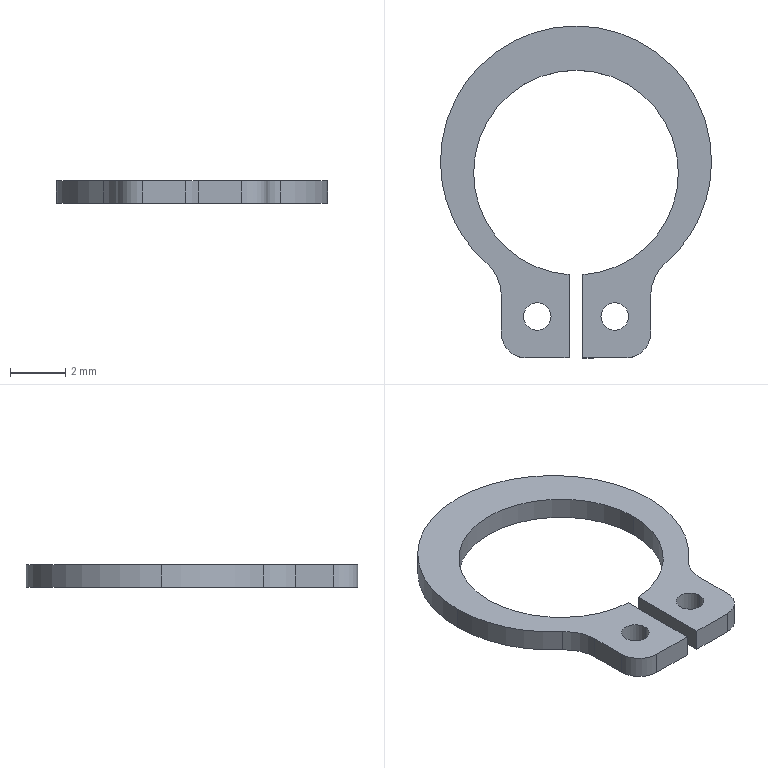Part | SolidWorks | features BaseBody 1 | 1 solid | 22 faces | box 9.8 x 12 x 0.8 mm | volume 33.948 mm3 | cylinder 14 | plane 8 | commonest cylinder face diameters 1 x4 7.4 x3 9.8 x3 1.8 x2 3 x2
STEP:
#1=CARTESIAN_POINT('',(-0.9,-5.2,-0.4));
#2=VERTEX_POINT('',#1);
#3=CARTESIAN_POINT('',(-1.9,-5.2,-0.4));
#4=VERTEX_POINT('',#3);
#5=CARTESIAN_POINT('',(-1.4,-5.2,-0.4));
#6=DIRECTION('',(0.,0.,-1.));
#7=DIRECTION('',(1.,0.,0.));
#8=AXIS2_PLACEMENT_3D('',#5,#6,#7);
#9=CIRCLE('',#8,0.5);
#10=EDGE_CURVE('',#2,#4,#9,.T.);
#11=ORIENTED_EDGE('',*,*,#10,.T.);
#12=CARTESIAN_POINT('',(-1.9,-5.2,0.4));
#13=VERTEX_POINT('',#12);
#14=CARTESIAN_POINT('',(-1.9,-5.2,0.4));
#15=DIRECTION('',(0.,0.,1.));
#16=VECTOR('',#15,1000.);
#17=LINE('',#14,#16);
#18=EDGE_CURVE('',#4,#13,#17,.T.);
#19=ORIENTED_EDGE('',*,*,#18,.T.);
#20=CARTESIAN_POINT('',(-0.9,-5.2,0.4));
#21=VERTEX_POINT('',#20);
#22=CARTESIAN_POINT('',(-1.4,-5.2,0.4));
#23=DIRECTION('',(0.,0.,-1.));
#24=DIRECTION('',(1.,0.,0.));
#25=AXIS2_PLACEMENT_3D('',#22,#23,#24);
#26=CIRCLE('',#25,0.5);
#27=EDGE_CURVE('',#21,#13,#26,.T.);
#28=ORIENTED_EDGE('',*,*,#27,.F.);
#29=CARTESIAN_POINT('',(-0.9,-5.2,0.4));
#30=DIRECTION('',(0.,0.,1.));
#31=VECTOR('',#30,1000.);
#32=LINE('',#29,#31);
#33=EDGE_CURVE('',#2,#21,#32,.T.);
#34=ORIENTED_EDGE('',*,*,#33,.F.);
#35=EDGE_LOOP('',(#11,#19,#28,#34));
#36=FACE_OUTER_BOUND('',#35,.T.);
#37=CARTESIAN_POINT('',(-1.4,-5.2,0.4));
#38=DIRECTION('',(0.,0.,1.));
#39=DIRECTION('',(1.,0.,0.));
#40=AXIS2_PLACEMENT_3D('',#37,#38,#39);
#41=CYLINDRICAL_SURFACE('',#40,0.5);
#42=ADVANCED_FACE('',(#36),#41,.F.);
#43=CARTESIAN_POINT('',(-0.25,-3.692,-0.4));
#44=VERTEX_POINT('',#43);
#45=CARTESIAN_POINT('',(-3.7,0.,-0.4));
#46=VERTEX_POINT('',#45);
#47=CARTESIAN_POINT('',(0.,0.,-0.4));
#48=DIRECTION('',(0.,0.,-1.));
#49=DIRECTION('',(1.,0.,0.));
#50=AXIS2_PLACEMENT_3D('',#47,#48,#49);
#51=CIRCLE('',#50,3.7);
#52=EDGE_CURVE('',#44,#46,#51,.T.);
#53=ORIENTED_EDGE('',*,*,#52,.T.);
#54=CARTESIAN_POINT('',(-3.7,0.,0.4));
#55=VERTEX_POINT('',#54);
#56=CARTESIAN_POINT('',(-3.7,0.,0.4));
#57=DIRECTION('',(0.,0.,1.));
#58=VECTOR('',#57,1000.);
#59=LINE('',#56,#58);
#60=EDGE_CURVE('',#46,#55,#59,.T.);
#61=ORIENTED_EDGE('',*,*,#60,.T.);
#62=CARTESIAN_POINT('',(-0.25,-3.692,0.4));
#63=VERTEX_POINT('',#62);
#64=CARTESIAN_POINT('',(0.,0.,0.4));
#65=DIRECTION('',(0.,0.,-1.));
#66=DIRECTION('',(1.,0.,0.));
#67=AXIS2_PLACEMENT_3D('',#64,#65,#66);
#68=CIRCLE('',#67,3.7);
#69=EDGE_CURVE('',#63,#55,#68,.T.);
#70=ORIENTED_EDGE('',*,*,#69,.F.);
#71=CARTESIAN_POINT('',(-0.25,-3.692,0.4));
#72=DIRECTION('',(0.,0.,1.));
#73=VECTOR('',#72,1000.);
#74=LINE('',#71,#73);
#75=EDGE_CURVE('',#44,#63,#74,.T.);
#76=ORIENTED_EDGE('',*,*,#75,.F.);
#77=EDGE_LOOP('',(#53,#61,#70,#76));
#78=FACE_OUTER_BOUND('',#77,.T.);
#79=CARTESIAN_POINT('',(0.,0.,0.4));
#80=DIRECTION('',(0.,0.,1.));
#81=DIRECTION('',(1.,0.,0.));
#82=AXIS2_PLACEMENT_3D('',#79,#80,#81);
#83=CYLINDRICAL_SURFACE('',#82,3.7);
#84=ADVANCED_FACE('',(#78),#83,.F.);
#85=ORIENTED_EDGE('',*,*,#60,.F.);
#86=CARTESIAN_POINT('',(3.7,0.,-0.4));
#87=VERTEX_POINT('',#86);
#88=CARTESIAN_POINT('',(0.,0.,-0.4));
#89=DIRECTION('',(0.,0.,-1.));
#90=DIRECTION('',(1.,0.,0.));
#91=AXIS2_PLACEMENT_3D('',#88,#89,#90);
#92=CIRCLE('',#91,3.7);
#93=EDGE_CURVE('',#46,#87,#92,.T.);
#94=ORIENTED_EDGE('',*,*,#93,.T.);
#95=CARTESIAN_POINT('',(3.7,0.,0.4));
#96=VERTEX_POINT('',#95);
#97=CARTESIAN_POINT('',(3.7,0.,0.4));
#98=DIRECTION('',(0.,0.,1.));
#99=VECTOR('',#98,1000.);
#100=LINE('',#97,#99);
#101=EDGE_CURVE('',#87,#96,#100,.T.);
#102=ORIENTED_EDGE('',*,*,#101,.T.);
#103=CARTESIAN_POINT('',(0.,0.,0.4));
#104=DIRECTION('',(0.,0.,-1.));
#105=DIRECTION('',(1.,0.,0.));
#106=AXIS2_PLACEMENT_3D('',#103,#104,#105);
#107=CIRCLE('',#106,3.7);
#108=EDGE_CURVE('',#55,#96,#107,.T.);
#109=ORIENTED_EDGE('',*,*,#108,.F.);
#110=EDGE_LOOP('',(#85,#94,#102,#109));
#111=FACE_OUTER_BOUND('',#110,.T.);
#112=CARTESIAN_POINT('',(0.,0.,0.4));
#113=DIRECTION('',(0.,0.,1.));
#114=DIRECTION('',(1.,0.,0.));
#115=AXIS2_PLACEMENT_3D('',#112,#113,#114);
#116=CYLINDRICAL_SURFACE('',#115,3.7);
#117=ADVANCED_FACE('',(#111),#116,.F.);
#118=CARTESIAN_POINT('',(4.9,0.4,-0.4));
#119=VERTEX_POINT('',#118);
#120=CARTESIAN_POINT('',(-4.9,0.4,-0.4));
#121=VERTEX_POINT('',#120);
#122=CARTESIAN_POINT('',(0.,0.4,-0.4));
#123=DIRECTION('',(0.,0.,1.));
#124=DIRECTION('',(1.,0.,0.));
#125=AXIS2_PLACEMENT_3D('',#122,#123,#124);
#126=CIRCLE('',#125,4.9);
#127=EDGE_CURVE('',#119,#121,#126,.T.);
#128=ORIENTED_EDGE('',*,*,#127,.T.);
#129=CARTESIAN_POINT('',(-4.9,0.4,0.4));
#130=VERTEX_POINT('',#129);
#131=CARTESIAN_POINT('',(-4.9,0.4,0.4));
#132=DIRECTION('',(0.,0.,1.));
#133=VECTOR('',#132,1000.);
#134=LINE('',#131,#133);
#135=EDGE_CURVE('',#121,#130,#134,.T.);
#136=ORIENTED_EDGE('',*,*,#135,.T.);
#137=CARTESIAN_POINT('',(4.9,0.4,0.4));
#138=VERTEX_POINT('',#137);
#139=CARTESIAN_POINT('',(0.,0.4,0.4));
#140=DIRECTION('',(0.,0.,-1.));
#141=DIRECTION('',(1.,0.,0.));
#142=AXIS2_PLACEMENT_3D('',#139,#140,#141);
#143=CIRCLE('',#142,4.9);
#144=EDGE_CURVE('',#130,#138,#143,.T.);
#145=ORIENTED_EDGE('',*,*,#144,.T.);
#146=CARTESIAN_POINT('',(4.9,0.4,0.4));
#147=DIRECTION('',(0.,0.,1.));
#148=VECTOR('',#147,1000.);
#149=LINE('',#146,#148);
#150=EDGE_CURVE('',#119,#138,#149,.T.);
#151=ORIENTED_EDGE('',*,*,#150,.F.);
#152=EDGE_LOOP('',(#128,#136,#145,#151));
#153=FACE_OUTER_BOUND('',#152,.T.);
#154=CARTESIAN_POINT('',(0.,0.4,0.4));
#155=DIRECTION('',(0.,0.,1.));
#156=DIRECTION('',(1.,0.,0.));
#157=AXIS2_PLACEMENT_3D('',#154,#155,#156);
#158=CYLINDRICAL_SURFACE('',#157,4.9);
#159=ADVANCED_FACE('',(#153),#158,.T.);
#160=CARTESIAN_POINT('',(3.216,-3.297,-0.4));
#161=VERTEX_POINT('',#160);
#162=CARTESIAN_POINT('',(0.,0.4,-0.4));
#163=DIRECTION('',(0.,0.,1.));
#164=DIRECTION('',(1.,0.,0.));
#165=AXIS2_PLACEMENT_3D('',#162,#163,#164);
#166=CIRCLE('',#165,4.9);
#167=EDGE_CURVE('',#161,#119,#166,.T.);
#168=ORIENTED_EDGE('',*,*,#167,.T.);
#169=ORIENTED_EDGE('',*,*,#150,.T.);
#170=CARTESIAN_POINT('',(3.216,-3.297,0.4));
#171=VERTEX_POINT('',#170);
#172=CARTESIAN_POINT('',(0.,0.4,0.4));
#173=DIRECTION('',(0.,0.,-1.));
#174=DIRECTION('',(1.,0.,0.));
#175=AXIS2_PLACEMENT_3D('',#172,#173,#174);
#176=CIRCLE('',#175,4.9);
#177=EDGE_CURVE('',#138,#171,#176,.T.);
#178=ORIENTED_EDGE('',*,*,#177,.T.);
#179=CARTESIAN_POINT('',(3.216,-3.297,0.4));
#180=DIRECTION('',(0.,0.,-1.));
#181=VECTOR('',#180,1000.);
#182=LINE('',#179,#181);
#183=EDGE_CURVE('',#171,#161,#182,.T.);
#184=ORIENTED_EDGE('',*,*,#183,.T.);
#185=EDGE_LOOP('',(#168,#169,#178,#184));
#186=FACE_OUTER_BOUND('',#185,.T.);
#187=CARTESIAN_POINT('',(0.,0.4,0.4));
#188=DIRECTION('',(0.,0.,1.));
#189=DIRECTION('',(1.,0.,0.));
#190=AXIS2_PLACEMENT_3D('',#187,#188,#189);
#191=CYLINDRICAL_SURFACE('',#190,4.9);
#192=ADVANCED_FACE('',(#186),#191,.T.);
#193=CARTESIAN_POINT('',(1.9,-5.2,-0.4));
#194=VERTEX_POINT('',#193);
#195=CARTESIAN_POINT('',(0.9,-5.2,-0.4));
#196=VERTEX_POINT('',#195);
#197=CARTESIAN_POINT('',(1.4,-5.2,-0.4));
#198=DIRECTION('',(0.,0.,-1.));
#199=DIRECTION('',(1.,0.,0.));
#200=AXIS2_PLACEMENT_3D('',#197,#198,#199);
#201=CIRCLE('',#200,0.5);
#202=EDGE_CURVE('',#194,#196,#201,.T.);
#203=ORIENTED_EDGE('',*,*,#202,.T.);
#204=CARTESIAN_POINT('',(0.9,-5.2,0.4));
#205=VERTEX_POINT('',#204);
#206=CARTESIAN_POINT('',(0.9,-5.2,0.4));
#207=DIRECTION('',(0.,0.,1.));
#208=VECTOR('',#207,1000.);
#209=LINE('',#206,#208);
#210=EDGE_CURVE('',#196,#205,#209,.T.);
#211=ORIENTED_EDGE('',*,*,#210,.T.);
#212=CARTESIAN_POINT('',(1.9,-5.2,0.4));
#213=VERTEX_POINT('',#212);
#214=CARTESIAN_POINT('',(1.4,-5.2,0.4));
#215=DIRECTION('',(0.,0.,-1.));
#216=DIRECTION('',(1.,0.,0.));
#217=AXIS2_PLACEMENT_3D('',#214,#215,#216);
#218=CIRCLE('',#217,0.5);
#219=EDGE_CURVE('',#213,#205,#218,.T.);
#220=ORIENTED_EDGE('',*,*,#219,.F.);
#221=CARTESIAN_POINT('',(1.9,-5.2,0.4));
#222=DIRECTION('',(0.,0.,1.));
#223=VECTOR('',#222,1000.);
#224=LINE('',#221,#223);
#225=EDGE_CURVE('',#194,#213,#224,.T.);
#226=ORIENTED_EDGE('',*,*,#225,.F.);
#227=EDGE_LOOP('',(#203,#211,#220,#226));
#228=FACE_OUTER_BOUND('',#227,.T.);
#229=CARTESIAN_POINT('',(1.4,-5.2,0.4));
#230=DIRECTION('',(0.,0.,1.));
#231=DIRECTION('',(1.,0.,0.));
#232=AXIS2_PLACEMENT_3D('',#229,#230,#231);
#233=CYLINDRICAL_SURFACE('',#232,0.5);
#234=ADVANCED_FACE('',(#228),#233,.F.);
#235=ORIENTED_EDGE('',*,*,#10,.F.);
#236=CARTESIAN_POINT('',(-1.4,-5.2,-0.4));
#237=DIRECTION('',(0.,0.,-1.));
#238=DIRECTION('',(1.,0.,0.));
#239=AXIS2_PLACEMENT_3D('',#236,#237,#238);
#240=CIRCLE('',#239,0.5);
#241=EDGE_CURVE('',#4,#2,#240,.T.);
#242=ORIENTED_EDGE('',*,*,#241,.F.);
#243=EDGE_LOOP('',(#235,#242));
#244=FACE_BOUND('',#243,.T.);
#245=CARTESIAN_POINT('',(2.7,-5.8,-0.4));
#246=VERTEX_POINT('',#245);
#247=CARTESIAN_POINT('',(2.7,-4.429,-0.4));
#248=VERTEX_POINT('',#247);
#249=CARTESIAN_POINT('',(2.7,-4.429,-0.4));
#250=DIRECTION('',(0.,1.,0.));
#251=VECTOR('',#250,1000.);
#252=LINE('',#249,#251);
#253=EDGE_CURVE('',#246,#248,#252,.T.);
#254=ORIENTED_EDGE('',*,*,#253,.F.);
#255=CARTESIAN_POINT('',(1.8,-6.7,-0.4));
#256=VERTEX_POINT('',#255);
#257=CARTESIAN_POINT('',(1.8,-5.8,-0.4));
#258=DIRECTION('',(0.,0.,1.));
#259=DIRECTION('',(1.,0.,0.));
#260=AXIS2_PLACEMENT_3D('',#257,#258,#259);
#261=CIRCLE('',#260,0.9);
#262=EDGE_CURVE('',#256,#246,#261,.T.);
#263=ORIENTED_EDGE('',*,*,#262,.F.);
#264=CARTESIAN_POINT('',(0.25,-6.7,-0.4));
#265=VERTEX_POINT('',#264);
#266=CARTESIAN_POINT('',(4.2,-6.7,-0.4));
#267=DIRECTION('',(1.,0.,0.));
#268=VECTOR('',#267,1000.);
#269=LINE('',#266,#268);
#270=EDGE_CURVE('',#265,#256,#269,.T.);
#271=ORIENTED_EDGE('',*,*,#270,.F.);
#272=CARTESIAN_POINT('',(0.25,-3.692,-0.4));
#273=VERTEX_POINT('',#272);
#274=CARTESIAN_POINT('',(0.25,-4.429,-0.4));
#275=DIRECTION('',(0.,-1.,0.));
#276=VECTOR('',#275,1000.);
#277=LINE('',#274,#276);
#278=EDGE_CURVE('',#273,#265,#277,.T.);
#279=ORIENTED_EDGE('',*,*,#278,.F.);
#280=CARTESIAN_POINT('',(0.,0.,-0.4));
#281=DIRECTION('',(0.,0.,-1.));
#282=DIRECTION('',(1.,0.,0.));
#283=AXIS2_PLACEMENT_3D('',#280,#281,#282);
#284=CIRCLE('',#283,3.7);
#285=EDGE_CURVE('',#87,#273,#284,.T.);
#286=ORIENTED_EDGE('',*,*,#285,.F.);
#287=ORIENTED_EDGE('',*,*,#93,.F.);
#288=ORIENTED_EDGE('',*,*,#52,.F.);
#289=CARTESIAN_POINT('',(-0.25,-6.7,-0.4));
#290=VERTEX_POINT('',#289);
#291=CARTESIAN_POINT('',(-0.25,-4.429,-0.4));
#292=DIRECTION('',(0.,1.,0.));
#293=VECTOR('',#292,1000.);
#294=LINE('',#291,#293);
#295=EDGE_CURVE('',#290,#44,#294,.T.);
#296=ORIENTED_EDGE('',*,*,#295,.F.);
#297=CARTESIAN_POINT('',(-1.8,-6.7,-0.4));
#298=VERTEX_POINT('',#297);
#299=CARTESIAN_POINT('',(4.2,-6.7,-0.4));
#300=DIRECTION('',(1.,0.,0.));
#301=VECTOR('',#300,1000.);
#302=LINE('',#299,#301);
#303=EDGE_CURVE('',#298,#290,#302,.T.);
#304=ORIENTED_EDGE('',*,*,#303,.F.);
#305=CARTESIAN_POINT('',(-2.7,-5.8,-0.4));
#306=VERTEX_POINT('',#305);
#307=CARTESIAN_POINT('',(-1.8,-5.8,-0.4));
#308=DIRECTION('',(0.,0.,1.));
#309=DIRECTION('',(1.,0.,0.));
#310=AXIS2_PLACEMENT_3D('',#307,#308,#309);
#311=CIRCLE('',#310,0.9);
#312=EDGE_CURVE('',#306,#298,#311,.T.);
#313=ORIENTED_EDGE('',*,*,#312,.F.);
#314=CARTESIAN_POINT('',(-2.7,-4.429,-0.4));
#315=VERTEX_POINT('',#314);
#316=CARTESIAN_POINT('',(-2.7,-4.429,-0.4));
#317=DIRECTION('',(0.,-1.,0.));
#318=VECTOR('',#317,1000.);
#319=LINE('',#316,#318);
#320=EDGE_CURVE('',#315,#306,#319,.T.);
#321=ORIENTED_EDGE('',*,*,#320,.F.);
#322=CARTESIAN_POINT('',(-3.216,-3.297,-0.4));
#323=VERTEX_POINT('',#322);
#324=CARTESIAN_POINT('',(-4.2,-4.429,-0.4));
#325=DIRECTION('',(0.,0.,-1.));
#326=DIRECTION('',(1.,0.,0.));
#327=AXIS2_PLACEMENT_3D('',#324,#325,#326);
#328=CIRCLE('',#327,1.5);
#329=EDGE_CURVE('',#323,#315,#328,.T.);
#330=ORIENTED_EDGE('',*,*,#329,.F.);
#331=CARTESIAN_POINT('',(0.,0.4,-0.4));
#332=DIRECTION('',(0.,0.,1.));
#333=DIRECTION('',(1.,0.,0.));
#334=AXIS2_PLACEMENT_3D('',#331,#332,#333);
#335=CIRCLE('',#334,4.9);
#336=EDGE_CURVE('',#121,#323,#335,.T.);
#337=ORIENTED_EDGE('',*,*,#336,.F.);
#338=ORIENTED_EDGE('',*,*,#127,.F.);
#339=ORIENTED_EDGE('',*,*,#167,.F.);
#340=CARTESIAN_POINT('',(4.2,-4.429,-0.4));
#341=DIRECTION('',(0.,0.,-1.));
#342=DIRECTION('',(1.,0.,0.));
#343=AXIS2_PLACEMENT_3D('',#340,#341,#342);
#344=CIRCLE('',#343,1.5);
#345=EDGE_CURVE('',#248,#161,#344,.T.);
#346=ORIENTED_EDGE('',*,*,#345,.F.);
#347=EDGE_LOOP('',(#254,#263,#271,#279,#286,#287,#288,#296,#304,#313,#321,#330,#337,#338,#339,#346));
#348=FACE_OUTER_BOUND('',#347,.T.);
#349=ORIENTED_EDGE('',*,*,#202,.F.);
#350=CARTESIAN_POINT('',(1.4,-5.2,-0.4));
#351=DIRECTION('',(0.,0.,-1.));
#352=DIRECTION('',(1.,0.,0.));
#353=AXIS2_PLACEMENT_3D('',#350,#351,#352);
#354=CIRCLE('',#353,0.5);
#355=EDGE_CURVE('',#196,#194,#354,.T.);
#356=ORIENTED_EDGE('',*,*,#355,.F.);
#357=EDGE_LOOP('',(#349,#356));
#358=FACE_BOUND('',#357,.T.);
#359=CARTESIAN_POINT('',(4.2,-4.429,-0.4));
#360=DIRECTION('',(0.,0.,1.));
#361=DIRECTION('',(1.,0.,0.));
#362=AXIS2_PLACEMENT_3D('',#359,#360,#361);
#363=PLANE('',#362);
#364=ADVANCED_FACE('',(#244,#348,#358),#363,.F.);
#365=ORIENTED_EDGE('',*,*,#18,.F.);
#366=ORIENTED_EDGE('',*,*,#241,.T.);
#367=ORIENTED_EDGE('',*,*,#33,.T.);
#368=CARTESIAN_POINT('',(-1.4,-5.2,0.4));
#369=DIRECTION('',(0.,0.,-1.));
#370=DIRECTION('',(1.,0.,0.));
#371=AXIS2_PLACEMENT_3D('',#368,#369,#370);
#372=CIRCLE('',#371,0.5);
#373=EDGE_CURVE('',#13,#21,#372,.T.);
#374=ORIENTED_EDGE('',*,*,#373,.F.);
#375=EDGE_LOOP('',(#365,#366,#367,#374));
#376=FACE_OUTER_BOUND('',#375,.T.);
#377=CARTESIAN_POINT('',(-1.4,-5.2,0.4));
#378=DIRECTION('',(0.,0.,1.));
#379=DIRECTION('',(1.,0.,0.));
#380=AXIS2_PLACEMENT_3D('',#377,#378,#379);
#381=CYLINDRICAL_SURFACE('',#380,0.5);
#382=ADVANCED_FACE('',(#376),#381,.F.);
#383=ORIENTED_EDGE('',*,*,#183,.F.);
#384=CARTESIAN_POINT('',(2.7,-4.429,0.4));
#385=VERTEX_POINT('',#384);
#386=CARTESIAN_POINT('',(4.2,-4.429,0.4));
#387=DIRECTION('',(0.,0.,-1.));
#388=DIRECTION('',(1.,0.,0.));
#389=AXIS2_PLACEMENT_3D('',#386,#387,#388);
#390=CIRCLE('',#389,1.5);
#391=EDGE_CURVE('',#385,#171,#390,.T.);
#392=ORIENTED_EDGE('',*,*,#391,.F.);
#393=CARTESIAN_POINT('',(2.7,-4.429,0.4));
#394=DIRECTION('',(0.,0.,1.));
#395=VECTOR('',#394,1000.);
#396=LINE('',#393,#395);
#397=EDGE_CURVE('',#248,#385,#396,.T.);
#398=ORIENTED_EDGE('',*,*,#397,.F.);
#399=ORIENTED_EDGE('',*,*,#345,.T.);
#400=EDGE_LOOP('',(#383,#392,#398,#399));
#401=FACE_OUTER_BOUND('',#400,.T.);
#402=CARTESIAN_POINT('',(4.2,-4.429,0.4));
#403=DIRECTION('',(0.,0.,1.));
#404=DIRECTION('',(1.,0.,0.));
#405=AXIS2_PLACEMENT_3D('',#402,#403,#404);
#406=CYLINDRICAL_SURFACE('',#405,1.5);
#407=ADVANCED_FACE('',(#401),#406,.F.);
#408=ORIENTED_EDGE('',*,*,#397,.T.);
#409=CARTESIAN_POINT('',(2.7,-5.8,0.4));
#410=VERTEX_POINT('',#409);
#411=CARTESIAN_POINT('',(2.7,-5.8,0.4));
#412=DIRECTION('',(0.,1.,0.));
#413=VECTOR('',#412,1000.);
#414=LINE('',#411,#413);
#415=EDGE_CURVE('',#410,#385,#414,.T.);
#416=ORIENTED_EDGE('',*,*,#415,.F.);
#417=CARTESIAN_POINT('',(2.7,-5.8,0.4));
#418=DIRECTION('',(0.,0.,1.));
#419=VECTOR('',#418,1000.);
#420=LINE('',#417,#419);
#421=EDGE_CURVE('',#246,#410,#420,.T.);
#422=ORIENTED_EDGE('',*,*,#421,.F.);
#423=ORIENTED_EDGE('',*,*,#253,.T.);
#424=EDGE_LOOP('',(#408,#416,#422,#423));
#425=FACE_OUTER_BOUND('',#424,.T.);
#426=CARTESIAN_POINT('',(2.7,-5.8,0.4));
#427=DIRECTION('',(-1.,0.,0.));
#428=DIRECTION('',(0.,0.,1.));
#429=AXIS2_PLACEMENT_3D('',#426,#427,#428);
#430=PLANE('',#429);
#431=ADVANCED_FACE('',(#425),#430,.F.);
#432=CARTESIAN_POINT('',(1.8,-6.7,0.4));
#433=VERTEX_POINT('',#432);
#434=CARTESIAN_POINT('',(1.8,-5.8,0.4));
#435=DIRECTION('',(0.,0.,-1.));
#436=DIRECTION('',(1.,0.,0.));
#437=AXIS2_PLACEMENT_3D('',#434,#435,#436);
#438=CIRCLE('',#437,0.9);
#439=EDGE_CURVE('',#410,#433,#438,.T.);
#440=ORIENTED_EDGE('',*,*,#439,.T.);
#441=CARTESIAN_POINT('',(1.8,-6.7,0.4));
#442=DIRECTION('',(0.,0.,-1.));
#443=VECTOR('',#442,1000.);
#444=LINE('',#441,#443);
#445=EDGE_CURVE('',#433,#256,#444,.T.);
#446=ORIENTED_EDGE('',*,*,#445,.T.);
#447=ORIENTED_EDGE('',*,*,#262,.T.);
#448=ORIENTED_EDGE('',*,*,#421,.T.);
#449=EDGE_LOOP('',(#440,#446,#447,#448));
#450=FACE_OUTER_BOUND('',#449,.T.);
#451=CARTESIAN_POINT('',(1.8,-5.8,0.4));
#452=DIRECTION('',(0.,0.,1.));
#453=DIRECTION('',(1.,0.,0.));
#454=AXIS2_PLACEMENT_3D('',#451,#452,#453);
#455=CYLINDRICAL_SURFACE('',#454,0.9);
#456=ADVANCED_FACE('',(#450),#455,.T.);
#457=ORIENTED_EDGE('',*,*,#445,.F.);
#458=CARTESIAN_POINT('',(0.25,-6.7,0.4));
#459=VERTEX_POINT('',#458);
#460=CARTESIAN_POINT('',(0.25,-6.7,0.4));
#461=DIRECTION('',(1.,0.,0.));
#462=VECTOR('',#461,1000.);
#463=LINE('',#460,#462);
#464=EDGE_CURVE('',#459,#433,#463,.T.);
#465=ORIENTED_EDGE('',*,*,#464,.F.);
#466=CARTESIAN_POINT('',(0.25,-6.7,0.4));
#467=DIRECTION('',(0.,0.,1.));
#468=VECTOR('',#467,1000.);
#469=LINE('',#466,#468);
#470=EDGE_CURVE('',#265,#459,#469,.T.);
#471=ORIENTED_EDGE('',*,*,#470,.F.);
#472=ORIENTED_EDGE('',*,*,#270,.T.);
#473=EDGE_LOOP('',(#457,#465,#471,#472));
#474=FACE_OUTER_BOUND('',#473,.T.);
#475=CARTESIAN_POINT('',(0.25,-6.7,0.4));
#476=DIRECTION('',(0.,1.,0.));
#477=DIRECTION('',(-1.,0.,0.));
#478=AXIS2_PLACEMENT_3D('',#475,#476,#477);
#479=PLANE('',#478);
#480=ADVANCED_FACE('',(#474),#479,.F.);
#481=ORIENTED_EDGE('',*,*,#470,.T.);
#482=CARTESIAN_POINT('',(0.25,-3.692,0.4));
#483=VERTEX_POINT('',#482);
#484=CARTESIAN_POINT('',(0.25,-3.692,0.4));
#485=DIRECTION('',(0.,-1.,0.));
#486=VECTOR('',#485,1000.);
#487=LINE('',#484,#486);
#488=EDGE_CURVE('',#483,#459,#487,.T.);
#489=ORIENTED_EDGE('',*,*,#488,.F.);
#490=CARTESIAN_POINT('',(0.25,-3.692,0.4));
#491=DIRECTION('',(0.,0.,1.));
#492=VECTOR('',#491,1000.);
#493=LINE('',#490,#492);
#494=EDGE_CURVE('',#273,#483,#493,.T.);
#495=ORIENTED_EDGE('',*,*,#494,.F.);
#496=ORIENTED_EDGE('',*,*,#278,.T.);
#497=EDGE_LOOP('',(#481,#489,#495,#496));
#498=FACE_OUTER_BOUND('',#497,.T.);
#499=CARTESIAN_POINT('',(0.25,-3.692,0.4));
#500=DIRECTION('',(1.,0.,0.));
#501=DIRECTION('',(0.,0.,-1.));
#502=AXIS2_PLACEMENT_3D('',#499,#500,#501);
#503=PLANE('',#502);
#504=ADVANCED_FACE('',(#498),#503,.F.);
#505=ORIENTED_EDGE('',*,*,#101,.F.);
#506=ORIENTED_EDGE('',*,*,#285,.T.);
#507=ORIENTED_EDGE('',*,*,#494,.T.);
#508=CARTESIAN_POINT('',(0.,0.,0.4));
#509=DIRECTION('',(0.,0.,-1.));
#510=DIRECTION('',(1.,0.,0.));
#511=AXIS2_PLACEMENT_3D('',#508,#509,#510);
#512=CIRCLE('',#511,3.7);
#513=EDGE_CURVE('',#96,#483,#512,.T.);
#514=ORIENTED_EDGE('',*,*,#513,.F.);
#515=EDGE_LOOP('',(#505,#506,#507,#514));
#516=FACE_OUTER_BOUND('',#515,.T.);
#517=CARTESIAN_POINT('',(0.,0.,0.4));
#518=DIRECTION('',(0.,0.,1.));
#519=DIRECTION('',(1.,0.,0.));
#520=AXIS2_PLACEMENT_3D('',#517,#518,#519);
#521=CYLINDRICAL_SURFACE('',#520,3.7);
#522=ADVANCED_FACE('',(#516),#521,.F.);
#523=ORIENTED_EDGE('',*,*,#75,.T.);
#524=CARTESIAN_POINT('',(-0.25,-6.7,0.4));
#525=VERTEX_POINT('',#524);
#526=CARTESIAN_POINT('',(-0.25,-6.7,0.4));
#527=DIRECTION('',(0.,1.,0.));
#528=VECTOR('',#527,1000.);
#529=LINE('',#526,#528);
#530=EDGE_CURVE('',#525,#63,#529,.T.);
#531=ORIENTED_EDGE('',*,*,#530,.F.);
#532=CARTESIAN_POINT('',(-0.25,-6.7,0.4));
#533=DIRECTION('',(0.,0.,1.));
#534=VECTOR('',#533,1000.);
#535=LINE('',#532,#534);
#536=EDGE_CURVE('',#290,#525,#535,.T.);
#537=ORIENTED_EDGE('',*,*,#536,.F.);
#538=ORIENTED_EDGE('',*,*,#295,.T.);
#539=EDGE_LOOP('',(#523,#531,#537,#538));
#540=FACE_OUTER_BOUND('',#539,.T.);
#541=CARTESIAN_POINT('',(-0.25,-6.7,0.4));
#542=DIRECTION('',(-1.,0.,0.));
#543=DIRECTION('',(0.,0.,1.));
#544=AXIS2_PLACEMENT_3D('',#541,#542,#543);
#545=PLANE('',#544);
#546=ADVANCED_FACE('',(#540),#545,.F.);
#547=ORIENTED_EDGE('',*,*,#536,.T.);
#548=CARTESIAN_POINT('',(-1.8,-6.7,0.4));
#549=VERTEX_POINT('',#548);
#550=CARTESIAN_POINT('',(-1.8,-6.7,0.4));
#551=DIRECTION('',(1.,0.,0.));
#552=VECTOR('',#551,1000.);
#553=LINE('',#550,#552);
#554=EDGE_CURVE('',#549,#525,#553,.T.);
#555=ORIENTED_EDGE('',*,*,#554,.F.);
#556=CARTESIAN_POINT('',(-1.8,-6.7,0.4));
#557=DIRECTION('',(0.,0.,1.));
#558=VECTOR('',#557,1000.);
#559=LINE('',#556,#558);
#560=EDGE_CURVE('',#298,#549,#559,.T.);
#561=ORIENTED_EDGE('',*,*,#560,.F.);
#562=ORIENTED_EDGE('',*,*,#303,.T.);
#563=EDGE_LOOP('',(#547,#555,#561,#562));
#564=FACE_OUTER_BOUND('',#563,.T.);
#565=CARTESIAN_POINT('',(-1.8,-6.7,0.4));
#566=DIRECTION('',(0.,1.,0.));
#567=DIRECTION('',(0.,0.,1.));
#568=AXIS2_PLACEMENT_3D('',#565,#566,#567);
#569=PLANE('',#568);
#570=ADVANCED_FACE('',(#564),#569,.F.);
#571=CARTESIAN_POINT('',(-2.7,-5.8,0.4));
#572=VERTEX_POINT('',#571);
#573=CARTESIAN_POINT('',(-1.8,-5.8,0.4));
#574=DIRECTION('',(0.,0.,-1.));
#575=DIRECTION('',(1.,0.,0.));
#576=AXIS2_PLACEMENT_3D('',#573,#574,#575);
#577=CIRCLE('',#576,0.9);
#578=EDGE_CURVE('',#549,#572,#577,.T.);
#579=ORIENTED_EDGE('',*,*,#578,.T.);
#580=CARTESIAN_POINT('',(-2.7,-5.8,0.4));
#581=DIRECTION('',(0.,0.,-1.));
#582=VECTOR('',#581,1000.);
#583=LINE('',#580,#582);
#584=EDGE_CURVE('',#572,#306,#583,.T.);
#585=ORIENTED_EDGE('',*,*,#584,.T.);
#586=ORIENTED_EDGE('',*,*,#312,.T.);
#587=ORIENTED_EDGE('',*,*,#560,.T.);
#588=EDGE_LOOP('',(#579,#585,#586,#587));
#589=FACE_OUTER_BOUND('',#588,.T.);
#590=CARTESIAN_POINT('',(-1.8,-5.8,0.4));
#591=DIRECTION('',(0.,0.,1.));
#592=DIRECTION('',(1.,0.,0.));
#593=AXIS2_PLACEMENT_3D('',#590,#591,#592);
#594=CYLINDRICAL_SURFACE('',#593,0.9);
#595=ADVANCED_FACE('',(#589),#594,.T.);
#596=ORIENTED_EDGE('',*,*,#584,.F.);
#597=CARTESIAN_POINT('',(-2.7,-4.429,0.4));
#598=VERTEX_POINT('',#597);
#599=CARTESIAN_POINT('',(-2.7,-4.429,0.4));
#600=DIRECTION('',(0.,-1.,0.));
#601=VECTOR('',#600,1000.);
#602=LINE('',#599,#601);
#603=EDGE_CURVE('',#598,#572,#602,.T.);
#604=ORIENTED_EDGE('',*,*,#603,.F.);
#605=CARTESIAN_POINT('',(-2.7,-4.429,0.4));
#606=DIRECTION('',(0.,0.,1.));
#607=VECTOR('',#606,1000.);
#608=LINE('',#605,#607);
#609=EDGE_CURVE('',#315,#598,#608,.T.);
#610=ORIENTED_EDGE('',*,*,#609,.F.);
#611=ORIENTED_EDGE('',*,*,#320,.T.);
#612=EDGE_LOOP('',(#596,#604,#610,#611));
#613=FACE_OUTER_BOUND('',#612,.T.);
#614=CARTESIAN_POINT('',(-2.7,-4.429,0.4));
#615=DIRECTION('',(1.,0.,0.));
#616=DIRECTION('',(0.,0.,-1.));
#617=AXIS2_PLACEMENT_3D('',#614,#615,#616);
#618=PLANE('',#617);
#619=ADVANCED_FACE('',(#613),#618,.F.);
#620=ORIENTED_EDGE('',*,*,#609,.T.);
#621=CARTESIAN_POINT('',(-3.216,-3.297,0.4));
#622=VERTEX_POINT('',#621);
#623=CARTESIAN_POINT('',(-4.2,-4.429,0.4));
#624=DIRECTION('',(0.,0.,-1.));
#625=DIRECTION('',(1.,0.,0.));
#626=AXIS2_PLACEMENT_3D('',#623,#624,#625);
#627=CIRCLE('',#626,1.5);
#628=EDGE_CURVE('',#622,#598,#627,.T.);
#629=ORIENTED_EDGE('',*,*,#628,.F.);
#630=CARTESIAN_POINT('',(-3.216,-3.297,0.4));
#631=DIRECTION('',(0.,0.,1.));
#632=VECTOR('',#631,1000.);
#633=LINE('',#630,#632);
#634=EDGE_CURVE('',#323,#622,#633,.T.);
#635=ORIENTED_EDGE('',*,*,#634,.F.);
#636=ORIENTED_EDGE('',*,*,#329,.T.);
#637=EDGE_LOOP('',(#620,#629,#635,#636));
#638=FACE_OUTER_BOUND('',#637,.T.);
#639=CARTESIAN_POINT('',(-4.2,-4.429,0.4));
#640=DIRECTION('',(0.,0.,1.));
#641=DIRECTION('',(1.,0.,0.));
#642=AXIS2_PLACEMENT_3D('',#639,#640,#641);
#643=CYLINDRICAL_SURFACE('',#642,1.5);
#644=ADVANCED_FACE('',(#638),#643,.F.);
#645=ORIENTED_EDGE('',*,*,#135,.F.);
#646=ORIENTED_EDGE('',*,*,#336,.T.);
#647=ORIENTED_EDGE('',*,*,#634,.T.);
#648=CARTESIAN_POINT('',(0.,0.4,0.4));
#649=DIRECTION('',(0.,0.,-1.));
#650=DIRECTION('',(1.,0.,0.));
#651=AXIS2_PLACEMENT_3D('',#648,#649,#650);
#652=CIRCLE('',#651,4.9);
#653=EDGE_CURVE('',#622,#130,#652,.T.);
#654=ORIENTED_EDGE('',*,*,#653,.T.);
#655=EDGE_LOOP('',(#645,#646,#647,#654));
#656=FACE_OUTER_BOUND('',#655,.T.);
#657=CARTESIAN_POINT('',(0.,0.4,0.4));
#658=DIRECTION('',(0.,0.,1.));
#659=DIRECTION('',(1.,0.,0.));
#660=AXIS2_PLACEMENT_3D('',#657,#658,#659);
#661=CYLINDRICAL_SURFACE('',#660,4.9);
#662=ADVANCED_FACE('',(#656),#661,.T.);
#663=ORIENTED_EDGE('',*,*,#210,.F.);
#664=ORIENTED_EDGE('',*,*,#355,.T.);
#665=ORIENTED_EDGE('',*,*,#225,.T.);
#666=CARTESIAN_POINT('',(1.4,-5.2,0.4));
#667=DIRECTION('',(0.,0.,-1.));
#668=DIRECTION('',(1.,0.,0.));
#669=AXIS2_PLACEMENT_3D('',#666,#667,#668);
#670=CIRCLE('',#669,0.5);
#671=EDGE_CURVE('',#205,#213,#670,.T.);
#672=ORIENTED_EDGE('',*,*,#671,.F.);
#673=EDGE_LOOP('',(#663,#664,#665,#672));
#674=FACE_OUTER_BOUND('',#673,.T.);
#675=CARTESIAN_POINT('',(1.4,-5.2,0.4));
#676=DIRECTION('',(0.,0.,1.));
#677=DIRECTION('',(1.,0.,0.));
#678=AXIS2_PLACEMENT_3D('',#675,#676,#677);
#679=CYLINDRICAL_SURFACE('',#678,0.5);
#680=ADVANCED_FACE('',(#674),#679,.F.);
#681=ORIENTED_EDGE('',*,*,#27,.T.);
#682=ORIENTED_EDGE('',*,*,#373,.T.);
#683=EDGE_LOOP('',(#681,#682));
#684=FACE_BOUND('',#683,.T.);
#685=ORIENTED_EDGE('',*,*,#439,.F.);
#686=ORIENTED_EDGE('',*,*,#415,.T.);
#687=ORIENTED_EDGE('',*,*,#391,.T.);
#688=ORIENTED_EDGE('',*,*,#177,.F.);
#689=ORIENTED_EDGE('',*,*,#144,.F.);
#690=ORIENTED_EDGE('',*,*,#653,.F.);
#691=ORIENTED_EDGE('',*,*,#628,.T.);
#692=ORIENTED_EDGE('',*,*,#603,.T.);
#693=ORIENTED_EDGE('',*,*,#578,.F.);
#694=ORIENTED_EDGE('',*,*,#554,.T.);
#695=ORIENTED_EDGE('',*,*,#530,.T.);
#696=ORIENTED_EDGE('',*,*,#69,.T.);
#697=ORIENTED_EDGE('',*,*,#108,.T.);
#698=ORIENTED_EDGE('',*,*,#513,.T.);
#699=ORIENTED_EDGE('',*,*,#488,.T.);
#700=ORIENTED_EDGE('',*,*,#464,.T.);
#701=EDGE_LOOP('',(#685,#686,#687,#688,#689,#690,#691,#692,#693,#694,#695,#696,#697,#698,#699,#700));
#702=FACE_OUTER_BOUND('',#701,.T.);
#703=ORIENTED_EDGE('',*,*,#219,.T.);
#704=ORIENTED_EDGE('',*,*,#671,.T.);
#705=EDGE_LOOP('',(#703,#704));
#706=FACE_BOUND('',#705,.T.);
#707=CARTESIAN_POINT('',(4.2,-4.429,0.4));
#708=DIRECTION('',(0.,0.,1.));
#709=DIRECTION('',(1.,0.,0.));
#710=AXIS2_PLACEMENT_3D('',#707,#708,#709);
#711=PLANE('',#710);
#712=ADVANCED_FACE('',(#684,#702,#706),#711,.T.);
#713=CLOSED_SHELL('',(#42,#84,#117,#159,#192,#234,#364,#382,#407,#431,#456,#480,#504,#522,#546,#570,#595,#619,#644,#662,#680,#712));
#714=MANIFOLD_SOLID_BREP('',#713);
#715=CARTESIAN_POINT('',(0.,0.,0.));
#716=DIRECTION('',(0.,0.,1.));
#717=DIRECTION('',(1.,0.,0.));
#718=AXIS2_PLACEMENT_3D('',#715,#716,#717);
#719=(LENGTH_UNIT()NAMED_UNIT(*)SI_UNIT(.MILLI.,.METRE.));
#720=UNCERTAINTY_MEASURE_WITH_UNIT(LENGTH_MEASURE(0.00001),#719,'','');
#721=(NAMED_UNIT(*)PLANE_ANGLE_UNIT()SI_UNIT($,.RADIAN.));
#722=(NAMED_UNIT(*)SI_UNIT($,.STERADIAN.)SOLID_ANGLE_UNIT());
#723=(GEOMETRIC_REPRESENTATION_CONTEXT(3)GLOBAL_UNCERTAINTY_ASSIGNED_CONTEXT((#720))GLOBAL_UNIT_ASSIGNED_CONTEXT((#719,#721,#722))REPRESENTATION_CONTEXT('',''));
#724=ADVANCED_BREP_SHAPE_REPRESENTATION('',(#714,#718),#723);